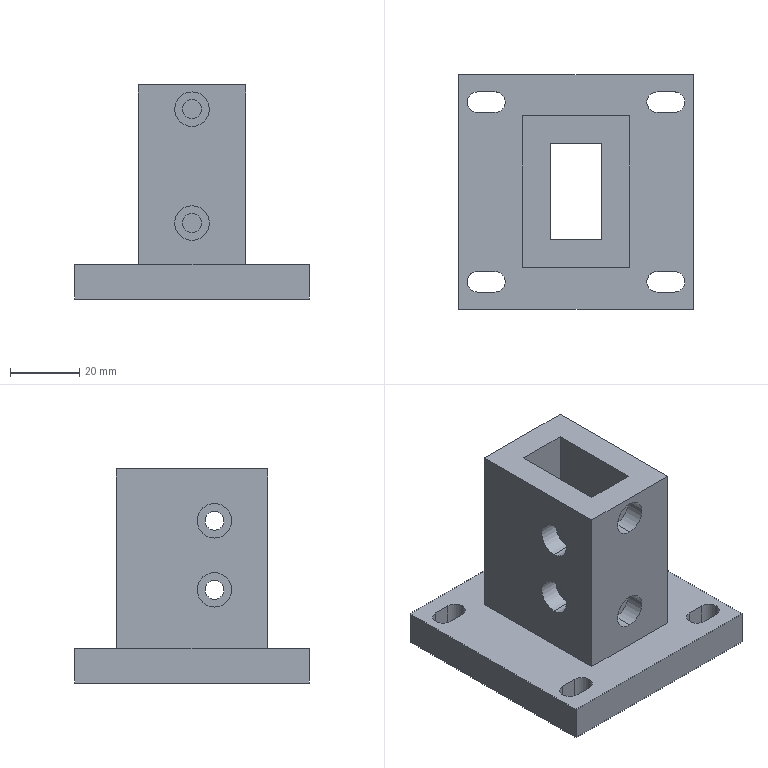Part | STEP file | X77-04401 | 1 solid | 65 faces | box 68 x 68 x 62 mm | volume 85783 mm3 | cylinder 36 | plane 29 | commonest cylinder face diameters 5.5 x12 6 x12 10 x12